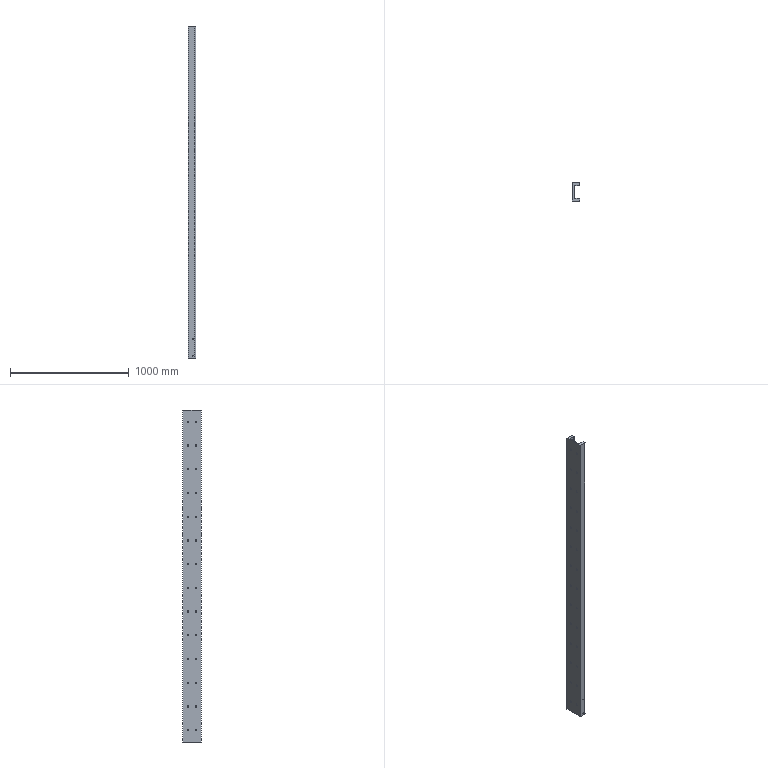Part | SolidWorks | features Fillet 2, ICE 2, Extrusion 1, HoleWzd 1 | 1 solid | 196 faces | box 61.2 x 157.2 x 2800 mm | volume 12681386 mm3 | cylinder 156 | plane 40 | commonest cylinder face diameters 11 x56 18 x56 5 x34 8.5 x8 12 x2